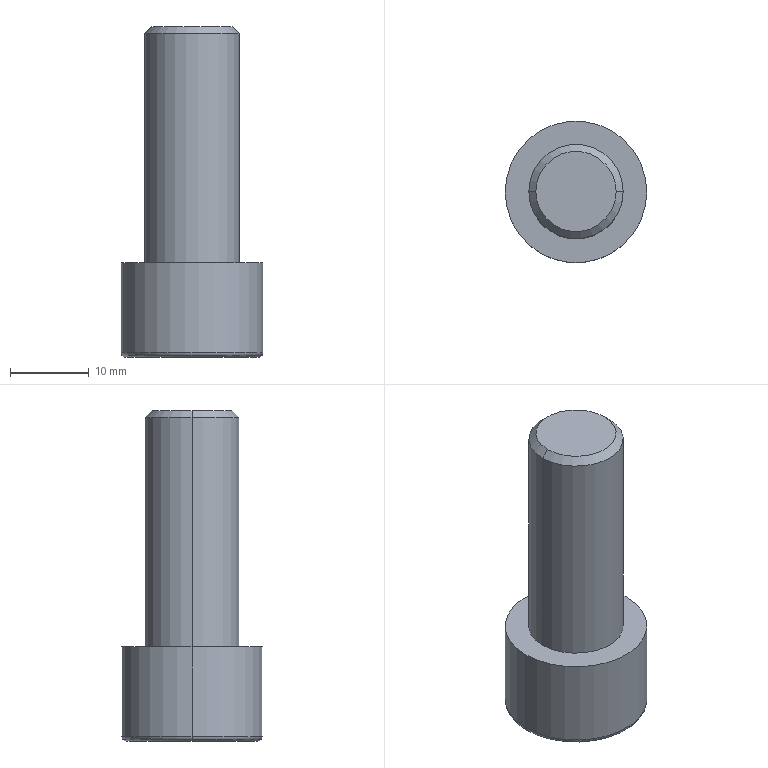Part | Creo | 1 solid | 20 faces | box 18 x 18 x 42 mm | volume 5742 mm3 | plane 10 | cylinder 4 | torus 4 | cone 2 | commonest cylinder face diameters 12 x2 18 x2
STEP:
#1=CARTESIAN_POINT('',(-191.,385.,-223.4));
#2=VERTEX_POINT('',#1);
#3=CARTESIAN_POINT('',(-179.,385.,-223.4));
#4=VERTEX_POINT('',#3);
#5=CARTESIAN_POINT('',(-185.,385.,-223.4));
#6=DIRECTION('',(0.,0.,1.));
#7=DIRECTION('',(-1.,0.,0.));
#8=AXIS2_PLACEMENT_3D('',#5,#6,#7);
#9=CIRCLE('',#8,6.);
#10=EDGE_CURVE('',#2,#4,#9,.T.);
#11=ORIENTED_EDGE('',*,*,#10,.T.);
#12=CARTESIAN_POINT('',(-179.,385.,-252.5));
#13=VERTEX_POINT('',#12);
#14=CARTESIAN_POINT('',(-179.,385.,-252.5));
#15=DIRECTION('',(0.,0.,1.));
#16=VECTOR('',#15,29.1);
#17=LINE('',#14,#16);
#18=EDGE_CURVE('',#13,#4,#17,.T.);
#19=ORIENTED_EDGE('',*,*,#18,.F.);
#20=CARTESIAN_POINT('',(-191.,385.,-252.5));
#21=VERTEX_POINT('',#20);
#22=CARTESIAN_POINT('',(-185.,385.,-252.5));
#23=DIRECTION('',(0.,0.,-1.));
#24=DIRECTION('',(1.,0.,0.));
#25=AXIS2_PLACEMENT_3D('',#22,#23,#24);
#26=CIRCLE('',#25,6.);
#27=EDGE_CURVE('',#13,#21,#26,.T.);
#28=ORIENTED_EDGE('',*,*,#27,.T.);
#29=CARTESIAN_POINT('',(-191.,385.,-252.5));
#30=DIRECTION('',(0.,0.,1.));
#31=VECTOR('',#30,29.1);
#32=LINE('',#29,#31);
#33=EDGE_CURVE('',#21,#2,#32,.T.);
#34=ORIENTED_EDGE('',*,*,#33,.T.);
#35=EDGE_LOOP('',(#11,#19,#28,#34));
#36=FACE_OUTER_BOUND('',#35,.F.);
#37=CARTESIAN_POINT('',(-185.,385.,-252.5));
#38=DIRECTION('',(0.,0.,1.));
#39=DIRECTION('',(-1.,0.,0.));
#40=AXIS2_PLACEMENT_3D('',#37,#38,#39);
#41=CYLINDRICAL_SURFACE('',#40,6.);
#42=ADVANCED_FACE('',(#36),#41,.T.);
#43=CARTESIAN_POINT('',(-190.1,385.,-222.5));
#44=VERTEX_POINT('',#43);
#45=CARTESIAN_POINT('',(-179.9,385.,-222.5));
#46=VERTEX_POINT('',#45);
#47=CARTESIAN_POINT('',(-185.,385.,-222.5));
#48=DIRECTION('',(0.,0.,1.));
#49=DIRECTION('',(-1.,0.,0.));
#50=AXIS2_PLACEMENT_3D('',#47,#48,#49);
#51=CIRCLE('',#50,5.1);
#52=EDGE_CURVE('',#44,#46,#51,.T.);
#53=ORIENTED_EDGE('',*,*,#52,.T.);
#54=CARTESIAN_POINT('',(-179.9,385.,-222.5));
#55=DIRECTION('',(0.7071,0.,-0.7071));
#56=VECTOR('',#55,1.273);
#57=LINE('',#54,#56);
#58=EDGE_CURVE('',#46,#4,#57,.T.);
#59=ORIENTED_EDGE('',*,*,#58,.T.);
#60=ORIENTED_EDGE('',*,*,#10,.F.);
#61=CARTESIAN_POINT('',(-190.1,385.,-222.5));
#62=DIRECTION('',(-0.7071,0.,-0.7071));
#63=VECTOR('',#62,1.273);
#64=LINE('',#61,#63);
#65=EDGE_CURVE('',#44,#2,#64,.T.);
#66=ORIENTED_EDGE('',*,*,#65,.F.);
#67=EDGE_LOOP('',(#53,#59,#60,#66));
#68=FACE_OUTER_BOUND('',#67,.F.);
#69=CARTESIAN_POINT('',(-185.,385.,-222.95));
#70=DIRECTION('',(0.,0.,-1.));
#71=DIRECTION('',(1.,0.,0.));
#72=AXIS2_PLACEMENT_3D('',#69,#70,#71);
#73=CONICAL_SURFACE('',#72,5.55,45.);
#74=ADVANCED_FACE('',(#68),#73,.T.);
#75=CARTESIAN_POINT('',(-185.,385.,-222.5));
#76=DIRECTION('',(0.,0.,1.));
#77=DIRECTION('',(1.,0.,0.));
#78=AXIS2_PLACEMENT_3D('',#75,#76,#77);
#79=CIRCLE('',#78,5.1);
#80=EDGE_CURVE('',#46,#44,#79,.T.);
#81=ORIENTED_EDGE('',*,*,#80,.F.);
#82=ORIENTED_EDGE('',*,*,#52,.F.);
#83=EDGE_LOOP('',(#81,#82));
#84=FACE_OUTER_BOUND('',#83,.F.);
#85=CARTESIAN_POINT('',(-185.,385.,-222.5));
#86=DIRECTION('',(0.,0.,-1.));
#87=DIRECTION('',(1.,0.,0.));
#88=AXIS2_PLACEMENT_3D('',#85,#86,#87);
#89=PLANE('',#88);
#90=ADVANCED_FACE('',(#84),#89,.F.);
#91=ORIENTED_EDGE('',*,*,#80,.T.);
#92=ORIENTED_EDGE('',*,*,#65,.T.);
#93=CARTESIAN_POINT('',(-185.,385.,-223.4));
#94=DIRECTION('',(0.,0.,1.));
#95=DIRECTION('',(1.,0.,0.));
#96=AXIS2_PLACEMENT_3D('',#93,#94,#95);
#97=CIRCLE('',#96,6.);
#98=EDGE_CURVE('',#4,#2,#97,.T.);
#99=ORIENTED_EDGE('',*,*,#98,.F.);
#100=ORIENTED_EDGE('',*,*,#58,.F.);
#101=EDGE_LOOP('',(#91,#92,#99,#100));
#102=FACE_OUTER_BOUND('',#101,.F.);
#103=CARTESIAN_POINT('',(-185.,385.,-222.95));
#104=DIRECTION('',(0.,0.,-1.));
#105=DIRECTION('',(1.,0.,0.));
#106=AXIS2_PLACEMENT_3D('',#103,#104,#105);
#107=CONICAL_SURFACE('',#106,5.55,45.);
#108=ADVANCED_FACE('',(#102),#107,.T.);
#109=ORIENTED_EDGE('',*,*,#98,.T.);
#110=ORIENTED_EDGE('',*,*,#33,.F.);
#111=CARTESIAN_POINT('',(-185.,385.,-252.5));
#112=DIRECTION('',(0.,0.,-1.));
#113=DIRECTION('',(-1.,0.,0.));
#114=AXIS2_PLACEMENT_3D('',#111,#112,#113);
#115=CIRCLE('',#114,6.);
#116=EDGE_CURVE('',#21,#13,#115,.T.);
#117=ORIENTED_EDGE('',*,*,#116,.T.);
#118=ORIENTED_EDGE('',*,*,#18,.T.);
#119=EDGE_LOOP('',(#109,#110,#117,#118));
#120=FACE_OUTER_BOUND('',#119,.F.);
#121=CARTESIAN_POINT('',(-185.,385.,-252.5));
#122=DIRECTION('',(0.,0.,1.));
#123=DIRECTION('',(-1.,0.,0.));
#124=AXIS2_PLACEMENT_3D('',#121,#122,#123);
#125=CYLINDRICAL_SURFACE('',#124,6.);
#126=ADVANCED_FACE('',(#120),#125,.T.);
#127=CARTESIAN_POINT('',(-176.,385.,-252.5));
#128=VERTEX_POINT('',#127);
#129=CARTESIAN_POINT('',(-194.,385.,-252.5));
#130=VERTEX_POINT('',#129);
#131=CARTESIAN_POINT('',(-185.,385.,-252.5));
#132=DIRECTION('',(0.,0.,1.));
#133=DIRECTION('',(1.,0.,0.));
#134=AXIS2_PLACEMENT_3D('',#131,#132,#133);
#135=CIRCLE('',#134,9.);
#136=EDGE_CURVE('',#128,#130,#135,.T.);
#137=ORIENTED_EDGE('',*,*,#136,.F.);
#138=CARTESIAN_POINT('',(-185.,385.,-252.5));
#139=DIRECTION('',(0.,0.,1.));
#140=DIRECTION('',(-1.,0.,0.));
#141=AXIS2_PLACEMENT_3D('',#138,#139,#140);
#142=CIRCLE('',#141,9.);
#143=EDGE_CURVE('',#130,#128,#142,.T.);
#144=ORIENTED_EDGE('',*,*,#143,.F.);
#145=EDGE_LOOP('',(#137,#144));
#146=FACE_OUTER_BOUND('',#145,.F.);
#147=ORIENTED_EDGE('',*,*,#27,.F.);
#148=ORIENTED_EDGE('',*,*,#116,.F.);
#149=EDGE_LOOP('',(#147,#148));
#150=FACE_BOUND('',#149,.F.);
#151=CARTESIAN_POINT('',(-185.,385.,-252.5));
#152=DIRECTION('',(0.,0.,1.));
#153=DIRECTION('',(-1.,0.,0.));
#154=AXIS2_PLACEMENT_3D('',#151,#152,#153);
#155=PLANE('',#154);
#156=ADVANCED_FACE('',(#146,#150),#155,.T.);
#157=CARTESIAN_POINT('',(-194.,385.,-263.9));
#158=VERTEX_POINT('',#157);
#159=CARTESIAN_POINT('',(-176.,385.,-263.9));
#160=VERTEX_POINT('',#159);
#161=CARTESIAN_POINT('',(-185.,385.,-263.9));
#162=DIRECTION('',(0.,0.,-1.));
#163=DIRECTION('',(-1.,0.,0.));
#164=AXIS2_PLACEMENT_3D('',#161,#162,#163);
#165=CIRCLE('',#164,9.);
#166=EDGE_CURVE('',#158,#160,#165,.T.);
#167=ORIENTED_EDGE('',*,*,#166,.T.);
#168=CARTESIAN_POINT('',(-176.,385.,-252.5));
#169=DIRECTION('',(0.,0.,-1.));
#170=VECTOR('',#169,11.4);
#171=LINE('',#168,#170);
#172=EDGE_CURVE('',#128,#160,#171,.T.);
#173=ORIENTED_EDGE('',*,*,#172,.F.);
#174=ORIENTED_EDGE('',*,*,#136,.T.);
#175=CARTESIAN_POINT('',(-194.,385.,-252.5));
#176=DIRECTION('',(0.,0.,-1.));
#177=VECTOR('',#176,11.4);
#178=LINE('',#175,#177);
#179=EDGE_CURVE('',#130,#158,#178,.T.);
#180=ORIENTED_EDGE('',*,*,#179,.T.);
#181=EDGE_LOOP('',(#167,#173,#174,#180));
#182=FACE_OUTER_BOUND('',#181,.F.);
#183=CARTESIAN_POINT('',(-185.,385.,-252.5));
#184=DIRECTION('',(0.,0.,-1.));
#185=DIRECTION('',(1.,0.,0.));
#186=AXIS2_PLACEMENT_3D('',#183,#184,#185);
#187=CYLINDRICAL_SURFACE('',#186,9.);
#188=ADVANCED_FACE('',(#182),#187,.T.);
#189=ORIENTED_EDGE('',*,*,#166,.F.);
#190=CARTESIAN_POINT('',(-193.824,385.,-264.324));
#191=VERTEX_POINT('',#190);
#192=CARTESIAN_POINT('',(-193.4,385.,-263.9));
#193=DIRECTION('',(0.,-1.,0.));
#194=DIRECTION('',(-1.,0.,0.));
#195=AXIS2_PLACEMENT_3D('',#192,#193,#194);
#196=CIRCLE('',#195,0.6);
#197=EDGE_CURVE('',#158,#191,#196,.T.);
#198=ORIENTED_EDGE('',*,*,#197,.T.);
#199=CARTESIAN_POINT('',(-176.176,385.,-264.324));
#200=VERTEX_POINT('',#199);
#201=CARTESIAN_POINT('',(-185.,385.,-264.324));
#202=DIRECTION('',(0.,0.,-1.));
#203=DIRECTION('',(-1.,0.,0.));
#204=AXIS2_PLACEMENT_3D('',#201,#202,#203);
#205=CIRCLE('',#204,8.824);
#206=EDGE_CURVE('',#191,#200,#205,.T.);
#207=ORIENTED_EDGE('',*,*,#206,.T.);
#208=CARTESIAN_POINT('',(-176.6,385.,-263.9));
#209=DIRECTION('',(0.,1.,0.));
#210=DIRECTION('',(1.,0.,0.));
#211=AXIS2_PLACEMENT_3D('',#208,#209,#210);
#212=CIRCLE('',#211,0.6);
#213=EDGE_CURVE('',#160,#200,#212,.T.);
#214=ORIENTED_EDGE('',*,*,#213,.F.);
#215=EDGE_LOOP('',(#189,#198,#207,#214));
#216=FACE_OUTER_BOUND('',#215,.F.);
#217=CARTESIAN_POINT('',(-185.,385.,-263.9));
#218=DIRECTION('',(0.,0.,-1.));
#219=DIRECTION('',(1.,0.,0.));
#220=AXIS2_PLACEMENT_3D('',#217,#218,#219);
#221=TOROIDAL_SURFACE('',#220,8.4,0.6);
#222=ADVANCED_FACE('',(#216),#221,.T.);
#223=CARTESIAN_POINT('',(-185.,385.,-263.9));
#224=DIRECTION('',(0.,0.,-1.));
#225=DIRECTION('',(1.,0.,0.));
#226=AXIS2_PLACEMENT_3D('',#223,#224,#225);
#227=CIRCLE('',#226,9.);
#228=EDGE_CURVE('',#160,#158,#227,.T.);
#229=ORIENTED_EDGE('',*,*,#228,.F.);
#230=ORIENTED_EDGE('',*,*,#213,.T.);
#231=CARTESIAN_POINT('',(-185.,385.,-264.324));
#232=DIRECTION('',(0.,0.,-1.));
#233=DIRECTION('',(1.,0.,0.));
#234=AXIS2_PLACEMENT_3D('',#231,#232,#233);
#235=CIRCLE('',#234,8.824);
#236=EDGE_CURVE('',#200,#191,#235,.T.);
#237=ORIENTED_EDGE('',*,*,#236,.T.);
#238=ORIENTED_EDGE('',*,*,#197,.F.);
#239=EDGE_LOOP('',(#229,#230,#237,#238));
#240=FACE_OUTER_BOUND('',#239,.F.);
#241=CARTESIAN_POINT('',(-185.,385.,-263.9));
#242=DIRECTION('',(0.,0.,-1.));
#243=DIRECTION('',(1.,0.,0.));
#244=AXIS2_PLACEMENT_3D('',#241,#242,#243);
#245=TOROIDAL_SURFACE('',#244,8.4,0.6);
#246=ADVANCED_FACE('',(#240),#245,.T.);
#247=ORIENTED_EDGE('',*,*,#228,.T.);
#248=ORIENTED_EDGE('',*,*,#179,.F.);
#249=ORIENTED_EDGE('',*,*,#143,.T.);
#250=ORIENTED_EDGE('',*,*,#172,.T.);
#251=EDGE_LOOP('',(#247,#248,#249,#250));
#252=FACE_OUTER_BOUND('',#251,.F.);
#253=CARTESIAN_POINT('',(-185.,385.,-252.5));
#254=DIRECTION('',(0.,0.,-1.));
#255=DIRECTION('',(1.,0.,0.));
#256=AXIS2_PLACEMENT_3D('',#253,#254,#255);
#257=CYLINDRICAL_SURFACE('',#256,9.);
#258=ADVANCED_FACE('',(#252),#257,.T.);
#259=CARTESIAN_POINT('',(-176.6,385.,-264.5));
#260=VERTEX_POINT('',#259);
#261=CARTESIAN_POINT('',(-193.4,385.,-264.5));
#262=VERTEX_POINT('',#261);
#263=CARTESIAN_POINT('',(-185.,385.,-264.5));
#264=DIRECTION('',(0.,0.,-1.));
#265=DIRECTION('',(1.,0.,0.));
#266=AXIS2_PLACEMENT_3D('',#263,#264,#265);
#267=CIRCLE('',#266,8.4);
#268=EDGE_CURVE('',#260,#262,#267,.T.);
#269=ORIENTED_EDGE('',*,*,#268,.T.);
#270=CARTESIAN_POINT('',(-193.4,385.,-263.9));
#271=DIRECTION('',(0.,-1.,0.));
#272=DIRECTION('',(-0.7071,0.,-0.7071));
#273=AXIS2_PLACEMENT_3D('',#270,#271,#272);
#274=CIRCLE('',#273,0.6);
#275=EDGE_CURVE('',#191,#262,#274,.T.);
#276=ORIENTED_EDGE('',*,*,#275,.F.);
#277=ORIENTED_EDGE('',*,*,#236,.F.);
#278=CARTESIAN_POINT('',(-176.6,385.,-263.9));
#279=DIRECTION('',(0.,1.,0.));
#280=DIRECTION('',(0.7071,0.,-0.7071));
#281=AXIS2_PLACEMENT_3D('',#278,#279,#280);
#282=CIRCLE('',#281,0.6);
#283=EDGE_CURVE('',#200,#260,#282,.T.);
#284=ORIENTED_EDGE('',*,*,#283,.T.);
#285=EDGE_LOOP('',(#269,#276,#277,#284));
#286=FACE_OUTER_BOUND('',#285,.F.);
#287=CARTESIAN_POINT('',(-185.,385.,-263.9));
#288=DIRECTION('',(0.,0.,-1.));
#289=DIRECTION('',(1.,0.,0.));
#290=AXIS2_PLACEMENT_3D('',#287,#288,#289);
#291=TOROIDAL_SURFACE('',#290,8.4,0.6);
#292=ADVANCED_FACE('',(#286),#291,.T.);
#293=ORIENTED_EDGE('',*,*,#268,.F.);
#294=CARTESIAN_POINT('',(-185.,385.,-264.5));
#295=DIRECTION('',(0.,0.,-1.));
#296=DIRECTION('',(-1.,0.,0.));
#297=AXIS2_PLACEMENT_3D('',#294,#295,#296);
#298=CIRCLE('',#297,8.4);
#299=EDGE_CURVE('',#262,#260,#298,.T.);
#300=ORIENTED_EDGE('',*,*,#299,.F.);
#301=EDGE_LOOP('',(#293,#300));
#302=FACE_OUTER_BOUND('',#301,.F.);
#303=CARTESIAN_POINT('',(-182.113,390.,-264.5));
#304=VERTEX_POINT('',#303);
#305=CARTESIAN_POINT('',(-187.887,390.,-264.5));
#306=VERTEX_POINT('',#305);
#307=CARTESIAN_POINT('',(-182.113,390.,-264.5));
#308=DIRECTION('',(-1.,0.,0.));
#309=VECTOR('',#308,5.774);
#310=LINE('',#307,#309);
#311=EDGE_CURVE('',#304,#306,#310,.T.);
#312=ORIENTED_EDGE('',*,*,#311,.F.);
#313=CARTESIAN_POINT('',(-179.226,385.,-264.5));
#314=VERTEX_POINT('',#313);
#315=CARTESIAN_POINT('',(-179.226,385.,-264.5));
#316=DIRECTION('',(-0.5,0.866,0.));
#317=VECTOR('',#316,5.774);
#318=LINE('',#315,#317);
#319=EDGE_CURVE('',#314,#304,#318,.T.);
#320=ORIENTED_EDGE('',*,*,#319,.F.);
#321=CARTESIAN_POINT('',(-182.113,380.,-264.5));
#322=VERTEX_POINT('',#321);
#323=CARTESIAN_POINT('',(-182.113,380.,-264.5));
#324=DIRECTION('',(0.5,0.866,0.));
#325=VECTOR('',#324,5.774);
#326=LINE('',#323,#325);
#327=EDGE_CURVE('',#322,#314,#326,.T.);
#328=ORIENTED_EDGE('',*,*,#327,.F.);
#329=CARTESIAN_POINT('',(-187.887,380.,-264.5));
#330=VERTEX_POINT('',#329);
#331=CARTESIAN_POINT('',(-187.887,380.,-264.5));
#332=DIRECTION('',(1.,0.,0.));
#333=VECTOR('',#332,5.774);
#334=LINE('',#331,#333);
#335=EDGE_CURVE('',#330,#322,#334,.T.);
#336=ORIENTED_EDGE('',*,*,#335,.F.);
#337=CARTESIAN_POINT('',(-190.774,385.,-264.5));
#338=VERTEX_POINT('',#337);
#339=CARTESIAN_POINT('',(-190.774,385.,-264.5));
#340=DIRECTION('',(0.5,-0.866,0.));
#341=VECTOR('',#340,5.774);
#342=LINE('',#339,#341);
#343=EDGE_CURVE('',#338,#330,#342,.T.);
#344=ORIENTED_EDGE('',*,*,#343,.F.);
#345=CARTESIAN_POINT('',(-187.887,390.,-264.5));
#346=DIRECTION('',(-0.5,-0.866,0.));
#347=VECTOR('',#346,5.774);
#348=LINE('',#345,#347);
#349=EDGE_CURVE('',#306,#338,#348,.T.);
#350=ORIENTED_EDGE('',*,*,#349,.F.);
#351=EDGE_LOOP('',(#312,#320,#328,#336,#344,#350));
#352=FACE_BOUND('',#351,.F.);
#353=CARTESIAN_POINT('',(-185.,385.,-264.5));
#354=DIRECTION('',(0.,0.,-1.));
#355=DIRECTION('',(1.,0.,0.));
#356=AXIS2_PLACEMENT_3D('',#353,#354,#355);
#357=PLANE('',#356);
#358=ADVANCED_FACE('',(#302,#352),#357,.T.);
#359=ORIENTED_EDGE('',*,*,#299,.T.);
#360=ORIENTED_EDGE('',*,*,#283,.F.);
#361=ORIENTED_EDGE('',*,*,#206,.F.);
#362=ORIENTED_EDGE('',*,*,#275,.T.);
#363=EDGE_LOOP('',(#359,#360,#361,#362));
#364=FACE_OUTER_BOUND('',#363,.F.);
#365=CARTESIAN_POINT('',(-185.,385.,-263.9));
#366=DIRECTION('',(0.,0.,-1.));
#367=DIRECTION('',(1.,0.,0.));
#368=AXIS2_PLACEMENT_3D('',#365,#366,#367);
#369=TOROIDAL_SURFACE('',#368,8.4,0.6);
#370=ADVANCED_FACE('',(#364),#369,.T.);
#371=ORIENTED_EDGE('',*,*,#311,.T.);
#372=CARTESIAN_POINT('',(-187.887,390.,-256.58));
#373=VERTEX_POINT('',#372);
#374=CARTESIAN_POINT('',(-187.887,390.,-264.5));
#375=DIRECTION('',(0.,0.,1.));
#376=VECTOR('',#375,7.92);
#377=LINE('',#374,#376);
#378=EDGE_CURVE('',#306,#373,#377,.T.);
#379=ORIENTED_EDGE('',*,*,#378,.T.);
#380=CARTESIAN_POINT('',(-182.113,390.,-256.58));
#381=VERTEX_POINT('',#380);
#382=CARTESIAN_POINT('',(-182.113,390.,-256.58));
#383=DIRECTION('',(-1.,0.,0.));
#384=VECTOR('',#383,5.774);
#385=LINE('',#382,#384);
#386=EDGE_CURVE('',#381,#373,#385,.T.);
#387=ORIENTED_EDGE('',*,*,#386,.F.);
#388=CARTESIAN_POINT('',(-182.113,390.,-264.5));
#389=DIRECTION('',(0.,0.,1.));
#390=VECTOR('',#389,7.92);
#391=LINE('',#388,#390);
#392=EDGE_CURVE('',#304,#381,#391,.T.);
#393=ORIENTED_EDGE('',*,*,#392,.F.);
#394=EDGE_LOOP('',(#371,#379,#387,#393));
#395=FACE_OUTER_BOUND('',#394,.F.);
#396=CARTESIAN_POINT('',(-187.887,390.,-256.58));
#397=DIRECTION('',(0.,1.,0.));
#398=DIRECTION('',(0.,0.,1.));
#399=AXIS2_PLACEMENT_3D('',#396,#397,#398);
#400=PLANE('',#399);
#401=ADVANCED_FACE('',(#395),#400,.F.);
#402=ORIENTED_EDGE('',*,*,#349,.T.);
#403=CARTESIAN_POINT('',(-190.774,385.,-256.58));
#404=VERTEX_POINT('',#403);
#405=CARTESIAN_POINT('',(-190.774,385.,-264.5));
#406=DIRECTION('',(0.,0.,1.));
#407=VECTOR('',#406,7.92);
#408=LINE('',#405,#407);
#409=EDGE_CURVE('',#338,#404,#408,.T.);
#410=ORIENTED_EDGE('',*,*,#409,.T.);
#411=CARTESIAN_POINT('',(-190.774,385.,-256.58));
#412=DIRECTION('',(0.5,0.866,0.));
#413=VECTOR('',#412,5.774);
#414=LINE('',#411,#413);
#415=EDGE_CURVE('',#404,#373,#414,.T.);
#416=ORIENTED_EDGE('',*,*,#415,.T.);
#417=ORIENTED_EDGE('',*,*,#378,.F.);
#418=EDGE_LOOP('',(#402,#410,#416,#417));
#419=FACE_OUTER_BOUND('',#418,.F.);
#420=CARTESIAN_POINT('',(-190.774,385.,-256.58));
#421=DIRECTION('',(-0.866,0.5,0.));
#422=DIRECTION('',(0.5,0.866,0.));
#423=AXIS2_PLACEMENT_3D('',#420,#421,#422);
#424=PLANE('',#423);
#425=ADVANCED_FACE('',(#419),#424,.F.);
#426=ORIENTED_EDGE('',*,*,#343,.T.);
#427=CARTESIAN_POINT('',(-187.887,380.,-256.58));
#428=VERTEX_POINT('',#427);
#429=CARTESIAN_POINT('',(-187.887,380.,-264.5));
#430=DIRECTION('',(0.,0.,1.));
#431=VECTOR('',#430,7.92);
#432=LINE('',#429,#431);
#433=EDGE_CURVE('',#330,#428,#432,.T.);
#434=ORIENTED_EDGE('',*,*,#433,.T.);
#435=CARTESIAN_POINT('',(-187.887,380.,-256.58));
#436=DIRECTION('',(-0.5,0.866,0.));
#437=VECTOR('',#436,5.774);
#438=LINE('',#435,#437);
#439=EDGE_CURVE('',#428,#404,#438,.T.);
#440=ORIENTED_EDGE('',*,*,#439,.T.);
#441=ORIENTED_EDGE('',*,*,#409,.F.);
#442=EDGE_LOOP('',(#426,#434,#440,#441));
#443=FACE_OUTER_BOUND('',#442,.F.);
#444=CARTESIAN_POINT('',(-187.887,380.,-256.58));
#445=DIRECTION('',(-0.866,-0.5,0.));
#446=DIRECTION('',(-0.5,0.866,0.));
#447=AXIS2_PLACEMENT_3D('',#444,#445,#446);
#448=PLANE('',#447);
#449=ADVANCED_FACE('',(#443),#448,.F.);
#450=ORIENTED_EDGE('',*,*,#335,.T.);
#451=CARTESIAN_POINT('',(-182.113,380.,-256.58));
#452=VERTEX_POINT('',#451);
#453=CARTESIAN_POINT('',(-182.113,380.,-264.5));
#454=DIRECTION('',(0.,0.,1.));
#455=VECTOR('',#454,7.92);
#456=LINE('',#453,#455);
#457=EDGE_CURVE('',#322,#452,#456,.T.);
#458=ORIENTED_EDGE('',*,*,#457,.T.);
#459=CARTESIAN_POINT('',(-187.887,380.,-256.58));
#460=DIRECTION('',(1.,0.,0.));
#461=VECTOR('',#460,5.774);
#462=LINE('',#459,#461);
#463=EDGE_CURVE('',#428,#452,#462,.T.);
#464=ORIENTED_EDGE('',*,*,#463,.F.);
#465=ORIENTED_EDGE('',*,*,#433,.F.);
#466=EDGE_LOOP('',(#450,#458,#464,#465));
#467=FACE_OUTER_BOUND('',#466,.F.);
#468=CARTESIAN_POINT('',(-182.113,380.,-256.58));
#469=DIRECTION('',(0.,-1.,0.));
#470=DIRECTION('',(0.,0.,-1.));
#471=AXIS2_PLACEMENT_3D('',#468,#469,#470);
#472=PLANE('',#471);
#473=ADVANCED_FACE('',(#467),#472,.F.);
#474=ORIENTED_EDGE('',*,*,#327,.T.);
#475=CARTESIAN_POINT('',(-179.226,385.,-256.58));
#476=VERTEX_POINT('',#475);
#477=CARTESIAN_POINT('',(-179.226,385.,-264.5));
#478=DIRECTION('',(0.,0.,1.));
#479=VECTOR('',#478,7.92);
#480=LINE('',#477,#479);
#481=EDGE_CURVE('',#314,#476,#480,.T.);
#482=ORIENTED_EDGE('',*,*,#481,.T.);
#483=CARTESIAN_POINT('',(-179.226,385.,-256.58));
#484=DIRECTION('',(-0.5,-0.866,0.));
#485=VECTOR('',#484,5.774);
#486=LINE('',#483,#485);
#487=EDGE_CURVE('',#476,#452,#486,.T.);
#488=ORIENTED_EDGE('',*,*,#487,.T.);
#489=ORIENTED_EDGE('',*,*,#457,.F.);
#490=EDGE_LOOP('',(#474,#482,#488,#489));
#491=FACE_OUTER_BOUND('',#490,.F.);
#492=CARTESIAN_POINT('',(-179.226,385.,-256.58));
#493=DIRECTION('',(0.866,-0.5,0.));
#494=DIRECTION('',(-0.5,-0.866,0.));
#495=AXIS2_PLACEMENT_3D('',#492,#493,#494);
#496=PLANE('',#495);
#497=ADVANCED_FACE('',(#491),#496,.F.);
#498=ORIENTED_EDGE('',*,*,#319,.T.);
#499=ORIENTED_EDGE('',*,*,#392,.T.);
#500=CARTESIAN_POINT('',(-182.113,390.,-256.58));
#501=DIRECTION('',(0.5,-0.866,0.));
#502=VECTOR('',#501,5.774);
#503=LINE('',#500,#502);
#504=EDGE_CURVE('',#381,#476,#503,.T.);
#505=ORIENTED_EDGE('',*,*,#504,.T.);
#506=ORIENTED_EDGE('',*,*,#481,.F.);
#507=EDGE_LOOP('',(#498,#499,#505,#506));
#508=FACE_OUTER_BOUND('',#507,.F.);
#509=CARTESIAN_POINT('',(-182.113,390.,-256.58));
#510=DIRECTION('',(0.866,0.5,0.));
#511=DIRECTION('',(0.5,-0.866,0.));
#512=AXIS2_PLACEMENT_3D('',#509,#510,#511);
#513=PLANE('',#512);
#514=ADVANCED_FACE('',(#508),#513,.F.);
#515=ORIENTED_EDGE('',*,*,#386,.T.);
#516=ORIENTED_EDGE('',*,*,#415,.F.);
#517=ORIENTED_EDGE('',*,*,#439,.F.);
#518=ORIENTED_EDGE('',*,*,#463,.T.);
#519=ORIENTED_EDGE('',*,*,#487,.F.);
#520=ORIENTED_EDGE('',*,*,#504,.F.);
#521=EDGE_LOOP('',(#515,#516,#517,#518,#519,#520));
#522=FACE_OUTER_BOUND('',#521,.F.);
#523=CARTESIAN_POINT('',(-182.113,390.,-256.58));
#524=DIRECTION('',(0.,0.,-1.));
#525=DIRECTION('',(1.,0.,0.));
#526=AXIS2_PLACEMENT_3D('',#523,#524,#525);
#527=PLANE('',#526);
#528=ADVANCED_FACE('',(#522),#527,.T.);
#529=CLOSED_SHELL('',(#42,#74,#90,#108,#126,#156,#188,#222,#246,#258,#292,#358,#370,#401,#425,#449,#473,#497,#514,#528));
#530=MANIFOLD_SOLID_BREP('',#529);
#531=(LENGTH_UNIT()NAMED_UNIT(*)SI_UNIT(.MILLI.,.METRE.));
#532=UNCERTAINTY_MEASURE_WITH_UNIT(LENGTH_MEASURE(0.004911),#531,'','');
#533=(NAMED_UNIT(*)PLANE_ANGLE_UNIT()SI_UNIT($,.RADIAN.));
#534=PLANE_ANGLE_MEASURE_WITH_UNIT(PLANE_ANGLE_MEASURE(0.01745),#533);
#535=(CONVERSION_BASED_UNIT('DEGREE',#534)NAMED_UNIT(*)PLANE_ANGLE_UNIT());
#536=(NAMED_UNIT(*)SI_UNIT($,.STERADIAN.)SOLID_ANGLE_UNIT());
#537=(GEOMETRIC_REPRESENTATION_CONTEXT(3)GLOBAL_UNCERTAINTY_ASSIGNED_CONTEXT((#532))GLOBAL_UNIT_ASSIGNED_CONTEXT((#531,#535,#536))REPRESENTATION_CONTEXT('',''));
#538=ADVANCED_BREP_SHAPE_REPRESENTATION('',(#530),#537);